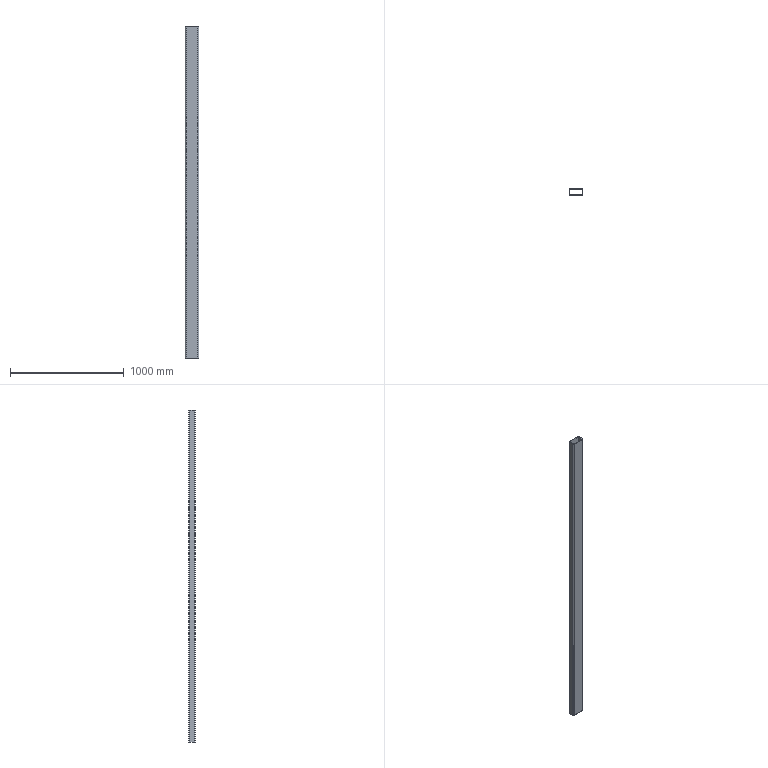Part | SolidWorks | features Extrusion 1 | 1 solid | 18 faces | box 120 x 60 x 2920 mm | volume 4776009 mm3 | plane 10 | cylinder 8 | commonest cylinder face diameters 10 x4 20 x4
STEP:
#1=CARTESIAN_POINT('',(110.,0.,2920.));
#2=VERTEX_POINT('',#1);
#3=CARTESIAN_POINT('',(120.,10.,2920.));
#4=VERTEX_POINT('',#3);
#5=CARTESIAN_POINT('',(110.,10.,2920.));
#6=DIRECTION('',(0.,0.,1.));
#7=DIRECTION('',(-1.,0.,0.));
#8=AXIS2_PLACEMENT_3D('',#5,#6,#7);
#9=CIRCLE('',#8,10.);
#10=EDGE_CURVE('',#2,#4,#9,.T.);
#11=ORIENTED_EDGE('',*,*,#10,.T.);
#12=CARTESIAN_POINT('',(120.,50.,2920.));
#13=VERTEX_POINT('',#12);
#14=CARTESIAN_POINT('',(120.,10.,2920.));
#15=DIRECTION('',(0.,1.,0.));
#16=VECTOR('',#15,1000.);
#17=LINE('',#14,#16);
#18=EDGE_CURVE('',#4,#13,#17,.T.);
#19=ORIENTED_EDGE('',*,*,#18,.T.);
#20=CARTESIAN_POINT('',(110.,60.,2920.));
#21=VERTEX_POINT('',#20);
#22=CARTESIAN_POINT('',(110.,50.,2920.));
#23=DIRECTION('',(0.,0.,1.));
#24=DIRECTION('',(1.,0.,0.));
#25=AXIS2_PLACEMENT_3D('',#22,#23,#24);
#26=CIRCLE('',#25,10.);
#27=EDGE_CURVE('',#13,#21,#26,.T.);
#28=ORIENTED_EDGE('',*,*,#27,.T.);
#29=CARTESIAN_POINT('',(10.,60.,2920.));
#30=VERTEX_POINT('',#29);
#31=CARTESIAN_POINT('',(10.,60.,2920.));
#32=DIRECTION('',(-1.,0.,0.));
#33=VECTOR('',#32,1000.);
#34=LINE('',#31,#33);
#35=EDGE_CURVE('',#21,#30,#34,.T.);
#36=ORIENTED_EDGE('',*,*,#35,.T.);
#37=CARTESIAN_POINT('',(0.,50.,2920.));
#38=VERTEX_POINT('',#37);
#39=CARTESIAN_POINT('',(10.,50.,2920.));
#40=DIRECTION('',(0.,0.,1.));
#41=DIRECTION('',(-1.,0.,0.));
#42=AXIS2_PLACEMENT_3D('',#39,#40,#41);
#43=CIRCLE('',#42,10.);
#44=EDGE_CURVE('',#30,#38,#43,.T.);
#45=ORIENTED_EDGE('',*,*,#44,.T.);
#46=CARTESIAN_POINT('',(0.,10.,2920.));
#47=VERTEX_POINT('',#46);
#48=CARTESIAN_POINT('',(0.,10.,2920.));
#49=DIRECTION('',(0.,-1.,0.));
#50=VECTOR('',#49,1000.);
#51=LINE('',#48,#50);
#52=EDGE_CURVE('',#38,#47,#51,.T.);
#53=ORIENTED_EDGE('',*,*,#52,.T.);
#54=CARTESIAN_POINT('',(10.,0.,2920.));
#55=VERTEX_POINT('',#54);
#56=CARTESIAN_POINT('',(10.,10.,2920.));
#57=DIRECTION('',(0.,0.,1.));
#58=DIRECTION('',(-1.,0.,0.));
#59=AXIS2_PLACEMENT_3D('',#56,#57,#58);
#60=CIRCLE('',#59,10.);
#61=EDGE_CURVE('',#47,#55,#60,.T.);
#62=ORIENTED_EDGE('',*,*,#61,.T.);
#63=CARTESIAN_POINT('',(10.,0.,2920.));
#64=DIRECTION('',(1.,0.,0.));
#65=VECTOR('',#64,1000.);
#66=LINE('',#63,#65);
#67=EDGE_CURVE('',#55,#2,#66,.T.);
#68=ORIENTED_EDGE('',*,*,#67,.T.);
#69=EDGE_LOOP('',(#11,#19,#28,#36,#45,#53,#62,#68));
#70=FACE_OUTER_BOUND('',#69,.T.);
#71=CARTESIAN_POINT('',(10.,55.,2920.));
#72=VERTEX_POINT('',#71);
#73=CARTESIAN_POINT('',(5.,50.,2920.));
#74=VERTEX_POINT('',#73);
#75=CARTESIAN_POINT('',(10.,50.,2920.));
#76=DIRECTION('',(0.,0.,1.));
#77=DIRECTION('',(-1.,0.,0.));
#78=AXIS2_PLACEMENT_3D('',#75,#76,#77);
#79=CIRCLE('',#78,5.);
#80=EDGE_CURVE('',#72,#74,#79,.T.);
#81=ORIENTED_EDGE('',*,*,#80,.F.);
#82=CARTESIAN_POINT('',(110.,55.,2920.));
#83=VERTEX_POINT('',#82);
#84=CARTESIAN_POINT('',(10.,55.,2920.));
#85=DIRECTION('',(-1.,0.,0.));
#86=VECTOR('',#85,1000.);
#87=LINE('',#84,#86);
#88=EDGE_CURVE('',#83,#72,#87,.T.);
#89=ORIENTED_EDGE('',*,*,#88,.F.);
#90=CARTESIAN_POINT('',(115.,50.,2920.));
#91=VERTEX_POINT('',#90);
#92=CARTESIAN_POINT('',(110.,50.,2920.));
#93=DIRECTION('',(0.,0.,1.));
#94=DIRECTION('',(1.,0.,0.));
#95=AXIS2_PLACEMENT_3D('',#92,#93,#94);
#96=CIRCLE('',#95,5.);
#97=EDGE_CURVE('',#91,#83,#96,.T.);
#98=ORIENTED_EDGE('',*,*,#97,.F.);
#99=CARTESIAN_POINT('',(115.,10.,2920.));
#100=VERTEX_POINT('',#99);
#101=CARTESIAN_POINT('',(115.,10.,2920.));
#102=DIRECTION('',(0.,1.,0.));
#103=VECTOR('',#102,1000.);
#104=LINE('',#101,#103);
#105=EDGE_CURVE('',#100,#91,#104,.T.);
#106=ORIENTED_EDGE('',*,*,#105,.F.);
#107=CARTESIAN_POINT('',(110.,5.,2920.));
#108=VERTEX_POINT('',#107);
#109=CARTESIAN_POINT('',(110.,10.,2920.));
#110=DIRECTION('',(0.,0.,1.));
#111=DIRECTION('',(-1.,0.,0.));
#112=AXIS2_PLACEMENT_3D('',#109,#110,#111);
#113=CIRCLE('',#112,5.);
#114=EDGE_CURVE('',#108,#100,#113,.T.);
#115=ORIENTED_EDGE('',*,*,#114,.F.);
#116=CARTESIAN_POINT('',(10.,5.,2920.));
#117=VERTEX_POINT('',#116);
#118=CARTESIAN_POINT('',(10.,5.,2920.));
#119=DIRECTION('',(1.,0.,0.));
#120=VECTOR('',#119,1000.);
#121=LINE('',#118,#120);
#122=EDGE_CURVE('',#117,#108,#121,.T.);
#123=ORIENTED_EDGE('',*,*,#122,.F.);
#124=CARTESIAN_POINT('',(5.,10.,2920.));
#125=VERTEX_POINT('',#124);
#126=CARTESIAN_POINT('',(10.,10.,2920.));
#127=DIRECTION('',(0.,0.,1.));
#128=DIRECTION('',(-1.,0.,0.));
#129=AXIS2_PLACEMENT_3D('',#126,#127,#128);
#130=CIRCLE('',#129,5.);
#131=EDGE_CURVE('',#125,#117,#130,.T.);
#132=ORIENTED_EDGE('',*,*,#131,.F.);
#133=CARTESIAN_POINT('',(5.,10.,2920.));
#134=DIRECTION('',(0.,-1.,0.));
#135=VECTOR('',#134,1000.);
#136=LINE('',#133,#135);
#137=EDGE_CURVE('',#74,#125,#136,.T.);
#138=ORIENTED_EDGE('',*,*,#137,.F.);
#139=EDGE_LOOP('',(#81,#89,#98,#106,#115,#123,#132,#138));
#140=FACE_BOUND('',#139,.T.);
#141=CARTESIAN_POINT('',(110.,10.,2920.));
#142=DIRECTION('',(0.,0.,-1.));
#143=DIRECTION('',(-1.,0.,0.));
#144=AXIS2_PLACEMENT_3D('',#141,#142,#143);
#145=PLANE('',#144);
#146=ADVANCED_FACE('',(#70,#140),#145,.F.);
#147=CARTESIAN_POINT('',(110.,0.,0.));
#148=VERTEX_POINT('',#147);
#149=CARTESIAN_POINT('',(120.,10.,0.));
#150=VERTEX_POINT('',#149);
#151=CARTESIAN_POINT('',(110.,10.,0.));
#152=DIRECTION('',(0.,0.,1.));
#153=DIRECTION('',(-1.,0.,0.));
#154=AXIS2_PLACEMENT_3D('',#151,#152,#153);
#155=CIRCLE('',#154,10.);
#156=EDGE_CURVE('',#148,#150,#155,.T.);
#157=ORIENTED_EDGE('',*,*,#156,.F.);
#158=CARTESIAN_POINT('',(10.,0.,0.));
#159=VERTEX_POINT('',#158);
#160=CARTESIAN_POINT('',(10.,0.,0.));
#161=DIRECTION('',(1.,0.,0.));
#162=VECTOR('',#161,1000.);
#163=LINE('',#160,#162);
#164=EDGE_CURVE('',#159,#148,#163,.T.);
#165=ORIENTED_EDGE('',*,*,#164,.F.);
#166=CARTESIAN_POINT('',(0.,10.,0.));
#167=VERTEX_POINT('',#166);
#168=CARTESIAN_POINT('',(10.,10.,0.));
#169=DIRECTION('',(0.,0.,1.));
#170=DIRECTION('',(-1.,0.,0.));
#171=AXIS2_PLACEMENT_3D('',#168,#169,#170);
#172=CIRCLE('',#171,10.);
#173=EDGE_CURVE('',#167,#159,#172,.T.);
#174=ORIENTED_EDGE('',*,*,#173,.F.);
#175=CARTESIAN_POINT('',(0.,50.,0.));
#176=VERTEX_POINT('',#175);
#177=CARTESIAN_POINT('',(0.,10.,0.));
#178=DIRECTION('',(0.,-1.,0.));
#179=VECTOR('',#178,1000.);
#180=LINE('',#177,#179);
#181=EDGE_CURVE('',#176,#167,#180,.T.);
#182=ORIENTED_EDGE('',*,*,#181,.F.);
#183=CARTESIAN_POINT('',(10.,60.,0.));
#184=VERTEX_POINT('',#183);
#185=CARTESIAN_POINT('',(10.,50.,0.));
#186=DIRECTION('',(0.,0.,1.));
#187=DIRECTION('',(-1.,0.,0.));
#188=AXIS2_PLACEMENT_3D('',#185,#186,#187);
#189=CIRCLE('',#188,10.);
#190=EDGE_CURVE('',#184,#176,#189,.T.);
#191=ORIENTED_EDGE('',*,*,#190,.F.);
#192=CARTESIAN_POINT('',(110.,60.,0.));
#193=VERTEX_POINT('',#192);
#194=CARTESIAN_POINT('',(10.,60.,0.));
#195=DIRECTION('',(-1.,0.,0.));
#196=VECTOR('',#195,1000.);
#197=LINE('',#194,#196);
#198=EDGE_CURVE('',#193,#184,#197,.T.);
#199=ORIENTED_EDGE('',*,*,#198,.F.);
#200=CARTESIAN_POINT('',(120.,50.,0.));
#201=VERTEX_POINT('',#200);
#202=CARTESIAN_POINT('',(110.,50.,0.));
#203=DIRECTION('',(0.,0.,1.));
#204=DIRECTION('',(1.,0.,0.));
#205=AXIS2_PLACEMENT_3D('',#202,#203,#204);
#206=CIRCLE('',#205,10.);
#207=EDGE_CURVE('',#201,#193,#206,.T.);
#208=ORIENTED_EDGE('',*,*,#207,.F.);
#209=CARTESIAN_POINT('',(120.,10.,0.));
#210=DIRECTION('',(0.,1.,0.));
#211=VECTOR('',#210,1000.);
#212=LINE('',#209,#211);
#213=EDGE_CURVE('',#150,#201,#212,.T.);
#214=ORIENTED_EDGE('',*,*,#213,.F.);
#215=EDGE_LOOP('',(#157,#165,#174,#182,#191,#199,#208,#214));
#216=FACE_OUTER_BOUND('',#215,.T.);
#217=CARTESIAN_POINT('',(110.,55.,0.));
#218=VERTEX_POINT('',#217);
#219=CARTESIAN_POINT('',(10.,55.,0.));
#220=VERTEX_POINT('',#219);
#221=CARTESIAN_POINT('',(10.,55.,0.));
#222=DIRECTION('',(-1.,0.,0.));
#223=VECTOR('',#222,1000.);
#224=LINE('',#221,#223);
#225=EDGE_CURVE('',#218,#220,#224,.T.);
#226=ORIENTED_EDGE('',*,*,#225,.T.);
#227=CARTESIAN_POINT('',(5.,50.,0.));
#228=VERTEX_POINT('',#227);
#229=CARTESIAN_POINT('',(10.,50.,0.));
#230=DIRECTION('',(0.,0.,1.));
#231=DIRECTION('',(-1.,0.,0.));
#232=AXIS2_PLACEMENT_3D('',#229,#230,#231);
#233=CIRCLE('',#232,5.);
#234=EDGE_CURVE('',#220,#228,#233,.T.);
#235=ORIENTED_EDGE('',*,*,#234,.T.);
#236=CARTESIAN_POINT('',(5.,10.,0.));
#237=VERTEX_POINT('',#236);
#238=CARTESIAN_POINT('',(5.,10.,0.));
#239=DIRECTION('',(0.,-1.,0.));
#240=VECTOR('',#239,1000.);
#241=LINE('',#238,#240);
#242=EDGE_CURVE('',#228,#237,#241,.T.);
#243=ORIENTED_EDGE('',*,*,#242,.T.);
#244=CARTESIAN_POINT('',(10.,5.,0.));
#245=VERTEX_POINT('',#244);
#246=CARTESIAN_POINT('',(10.,10.,0.));
#247=DIRECTION('',(0.,0.,1.));
#248=DIRECTION('',(-1.,0.,0.));
#249=AXIS2_PLACEMENT_3D('',#246,#247,#248);
#250=CIRCLE('',#249,5.);
#251=EDGE_CURVE('',#237,#245,#250,.T.);
#252=ORIENTED_EDGE('',*,*,#251,.T.);
#253=CARTESIAN_POINT('',(110.,5.,0.));
#254=VERTEX_POINT('',#253);
#255=CARTESIAN_POINT('',(10.,5.,0.));
#256=DIRECTION('',(1.,0.,0.));
#257=VECTOR('',#256,1000.);
#258=LINE('',#255,#257);
#259=EDGE_CURVE('',#245,#254,#258,.T.);
#260=ORIENTED_EDGE('',*,*,#259,.T.);
#261=CARTESIAN_POINT('',(115.,10.,0.));
#262=VERTEX_POINT('',#261);
#263=CARTESIAN_POINT('',(110.,10.,0.));
#264=DIRECTION('',(0.,0.,1.));
#265=DIRECTION('',(-1.,0.,0.));
#266=AXIS2_PLACEMENT_3D('',#263,#264,#265);
#267=CIRCLE('',#266,5.);
#268=EDGE_CURVE('',#254,#262,#267,.T.);
#269=ORIENTED_EDGE('',*,*,#268,.T.);
#270=CARTESIAN_POINT('',(115.,50.,0.));
#271=VERTEX_POINT('',#270);
#272=CARTESIAN_POINT('',(115.,10.,0.));
#273=DIRECTION('',(0.,1.,0.));
#274=VECTOR('',#273,1000.);
#275=LINE('',#272,#274);
#276=EDGE_CURVE('',#262,#271,#275,.T.);
#277=ORIENTED_EDGE('',*,*,#276,.T.);
#278=CARTESIAN_POINT('',(110.,50.,0.));
#279=DIRECTION('',(0.,0.,1.));
#280=DIRECTION('',(1.,0.,0.));
#281=AXIS2_PLACEMENT_3D('',#278,#279,#280);
#282=CIRCLE('',#281,5.);
#283=EDGE_CURVE('',#271,#218,#282,.T.);
#284=ORIENTED_EDGE('',*,*,#283,.T.);
#285=EDGE_LOOP('',(#226,#235,#243,#252,#260,#269,#277,#284));
#286=FACE_BOUND('',#285,.T.);
#287=CARTESIAN_POINT('',(110.,10.,0.));
#288=DIRECTION('',(0.,0.,-1.));
#289=DIRECTION('',(-1.,0.,0.));
#290=AXIS2_PLACEMENT_3D('',#287,#288,#289);
#291=PLANE('',#290);
#292=ADVANCED_FACE('',(#216,#286),#291,.T.);
#293=ORIENTED_EDGE('',*,*,#156,.T.);
#294=CARTESIAN_POINT('',(120.,10.,2920.));
#295=DIRECTION('',(0.,0.,-1.));
#296=VECTOR('',#295,1000.);
#297=LINE('',#294,#296);
#298=EDGE_CURVE('',#4,#150,#297,.T.);
#299=ORIENTED_EDGE('',*,*,#298,.F.);
#300=ORIENTED_EDGE('',*,*,#10,.F.);
#301=CARTESIAN_POINT('',(110.,0.,2920.));
#302=DIRECTION('',(0.,0.,-1.));
#303=VECTOR('',#302,1000.);
#304=LINE('',#301,#303);
#305=EDGE_CURVE('',#2,#148,#304,.T.);
#306=ORIENTED_EDGE('',*,*,#305,.T.);
#307=EDGE_LOOP('',(#293,#299,#300,#306));
#308=FACE_OUTER_BOUND('',#307,.T.);
#309=CARTESIAN_POINT('',(110.,10.,2920.));
#310=DIRECTION('',(0.,0.,-1.));
#311=DIRECTION('',(-1.,0.,0.));
#312=AXIS2_PLACEMENT_3D('',#309,#310,#311);
#313=CYLINDRICAL_SURFACE('',#312,10.);
#314=ADVANCED_FACE('',(#308),#313,.T.);
#315=ORIENTED_EDGE('',*,*,#213,.T.);
#316=CARTESIAN_POINT('',(120.,50.,2920.));
#317=DIRECTION('',(0.,0.,-1.));
#318=VECTOR('',#317,1000.);
#319=LINE('',#316,#318);
#320=EDGE_CURVE('',#13,#201,#319,.T.);
#321=ORIENTED_EDGE('',*,*,#320,.F.);
#322=ORIENTED_EDGE('',*,*,#18,.F.);
#323=ORIENTED_EDGE('',*,*,#298,.T.);
#324=EDGE_LOOP('',(#315,#321,#322,#323));
#325=FACE_OUTER_BOUND('',#324,.T.);
#326=CARTESIAN_POINT('',(120.,10.,2920.));
#327=DIRECTION('',(-1.,0.,0.));
#328=DIRECTION('',(0.,-1.,0.));
#329=AXIS2_PLACEMENT_3D('',#326,#327,#328);
#330=PLANE('',#329);
#331=ADVANCED_FACE('',(#325),#330,.F.);
#332=ORIENTED_EDGE('',*,*,#207,.T.);
#333=CARTESIAN_POINT('',(110.,60.,2920.));
#334=DIRECTION('',(0.,0.,-1.));
#335=VECTOR('',#334,1000.);
#336=LINE('',#333,#335);
#337=EDGE_CURVE('',#21,#193,#336,.T.);
#338=ORIENTED_EDGE('',*,*,#337,.F.);
#339=ORIENTED_EDGE('',*,*,#27,.F.);
#340=ORIENTED_EDGE('',*,*,#320,.T.);
#341=EDGE_LOOP('',(#332,#338,#339,#340));
#342=FACE_OUTER_BOUND('',#341,.T.);
#343=CARTESIAN_POINT('',(110.,50.,2920.));
#344=DIRECTION('',(0.,0.,-1.));
#345=DIRECTION('',(-1.,0.,0.));
#346=AXIS2_PLACEMENT_3D('',#343,#344,#345);
#347=CYLINDRICAL_SURFACE('',#346,10.);
#348=ADVANCED_FACE('',(#342),#347,.T.);
#349=ORIENTED_EDGE('',*,*,#198,.T.);
#350=CARTESIAN_POINT('',(10.,60.,2920.));
#351=DIRECTION('',(0.,0.,-1.));
#352=VECTOR('',#351,1000.);
#353=LINE('',#350,#352);
#354=EDGE_CURVE('',#30,#184,#353,.T.);
#355=ORIENTED_EDGE('',*,*,#354,.F.);
#356=ORIENTED_EDGE('',*,*,#35,.F.);
#357=ORIENTED_EDGE('',*,*,#337,.T.);
#358=EDGE_LOOP('',(#349,#355,#356,#357));
#359=FACE_OUTER_BOUND('',#358,.T.);
#360=CARTESIAN_POINT('',(10.,60.,2920.));
#361=DIRECTION('',(0.,-1.,0.));
#362=DIRECTION('',(0.,0.,-1.));
#363=AXIS2_PLACEMENT_3D('',#360,#361,#362);
#364=PLANE('',#363);
#365=ADVANCED_FACE('',(#359),#364,.F.);
#366=ORIENTED_EDGE('',*,*,#190,.T.);
#367=CARTESIAN_POINT('',(0.,50.,2920.));
#368=DIRECTION('',(0.,0.,-1.));
#369=VECTOR('',#368,1000.);
#370=LINE('',#367,#369);
#371=EDGE_CURVE('',#38,#176,#370,.T.);
#372=ORIENTED_EDGE('',*,*,#371,.F.);
#373=ORIENTED_EDGE('',*,*,#44,.F.);
#374=ORIENTED_EDGE('',*,*,#354,.T.);
#375=EDGE_LOOP('',(#366,#372,#373,#374));
#376=FACE_OUTER_BOUND('',#375,.T.);
#377=CARTESIAN_POINT('',(10.,50.,2920.));
#378=DIRECTION('',(0.,0.,-1.));
#379=DIRECTION('',(-1.,0.,0.));
#380=AXIS2_PLACEMENT_3D('',#377,#378,#379);
#381=CYLINDRICAL_SURFACE('',#380,10.);
#382=ADVANCED_FACE('',(#376),#381,.T.);
#383=ORIENTED_EDGE('',*,*,#181,.T.);
#384=CARTESIAN_POINT('',(0.,10.,2920.));
#385=DIRECTION('',(0.,0.,-1.));
#386=VECTOR('',#385,1000.);
#387=LINE('',#384,#386);
#388=EDGE_CURVE('',#47,#167,#387,.T.);
#389=ORIENTED_EDGE('',*,*,#388,.F.);
#390=ORIENTED_EDGE('',*,*,#52,.F.);
#391=ORIENTED_EDGE('',*,*,#371,.T.);
#392=EDGE_LOOP('',(#383,#389,#390,#391));
#393=FACE_OUTER_BOUND('',#392,.T.);
#394=CARTESIAN_POINT('',(0.,10.,2920.));
#395=DIRECTION('',(1.,0.,0.));
#396=DIRECTION('',(0.,1.,0.));
#397=AXIS2_PLACEMENT_3D('',#394,#395,#396);
#398=PLANE('',#397);
#399=ADVANCED_FACE('',(#393),#398,.F.);
#400=ORIENTED_EDGE('',*,*,#173,.T.);
#401=CARTESIAN_POINT('',(10.,0.,2920.));
#402=DIRECTION('',(0.,0.,-1.));
#403=VECTOR('',#402,1000.);
#404=LINE('',#401,#403);
#405=EDGE_CURVE('',#55,#159,#404,.T.);
#406=ORIENTED_EDGE('',*,*,#405,.F.);
#407=ORIENTED_EDGE('',*,*,#61,.F.);
#408=ORIENTED_EDGE('',*,*,#388,.T.);
#409=EDGE_LOOP('',(#400,#406,#407,#408));
#410=FACE_OUTER_BOUND('',#409,.T.);
#411=CARTESIAN_POINT('',(10.,10.,2920.));
#412=DIRECTION('',(0.,0.,-1.));
#413=DIRECTION('',(-1.,0.,0.));
#414=AXIS2_PLACEMENT_3D('',#411,#412,#413);
#415=CYLINDRICAL_SURFACE('',#414,10.);
#416=ADVANCED_FACE('',(#410),#415,.T.);
#417=ORIENTED_EDGE('',*,*,#164,.T.);
#418=ORIENTED_EDGE('',*,*,#305,.F.);
#419=ORIENTED_EDGE('',*,*,#67,.F.);
#420=ORIENTED_EDGE('',*,*,#405,.T.);
#421=EDGE_LOOP('',(#417,#418,#419,#420));
#422=FACE_OUTER_BOUND('',#421,.T.);
#423=CARTESIAN_POINT('',(10.,0.,2920.));
#424=DIRECTION('',(0.,1.,0.));
#425=DIRECTION('',(0.,0.,1.));
#426=AXIS2_PLACEMENT_3D('',#423,#424,#425);
#427=PLANE('',#426);
#428=ADVANCED_FACE('',(#422),#427,.F.);
#429=ORIENTED_EDGE('',*,*,#234,.F.);
#430=CARTESIAN_POINT('',(10.,55.,2920.));
#431=DIRECTION('',(0.,0.,-1.));
#432=VECTOR('',#431,1000.);
#433=LINE('',#430,#432);
#434=EDGE_CURVE('',#72,#220,#433,.T.);
#435=ORIENTED_EDGE('',*,*,#434,.F.);
#436=ORIENTED_EDGE('',*,*,#80,.T.);
#437=CARTESIAN_POINT('',(5.,50.,2920.));
#438=DIRECTION('',(0.,0.,-1.));
#439=VECTOR('',#438,1000.);
#440=LINE('',#437,#439);
#441=EDGE_CURVE('',#74,#228,#440,.T.);
#442=ORIENTED_EDGE('',*,*,#441,.T.);
#443=EDGE_LOOP('',(#429,#435,#436,#442));
#444=FACE_OUTER_BOUND('',#443,.T.);
#445=CARTESIAN_POINT('',(10.,50.,2920.));
#446=DIRECTION('',(0.,0.,-1.));
#447=DIRECTION('',(-1.,0.,0.));
#448=AXIS2_PLACEMENT_3D('',#445,#446,#447);
#449=CYLINDRICAL_SURFACE('',#448,5.);
#450=ADVANCED_FACE('',(#444),#449,.F.);
#451=ORIENTED_EDGE('',*,*,#242,.F.);
#452=ORIENTED_EDGE('',*,*,#441,.F.);
#453=ORIENTED_EDGE('',*,*,#137,.T.);
#454=CARTESIAN_POINT('',(5.,10.,2920.));
#455=DIRECTION('',(0.,0.,-1.));
#456=VECTOR('',#455,1000.);
#457=LINE('',#454,#456);
#458=EDGE_CURVE('',#125,#237,#457,.T.);
#459=ORIENTED_EDGE('',*,*,#458,.T.);
#460=EDGE_LOOP('',(#451,#452,#453,#459));
#461=FACE_OUTER_BOUND('',#460,.T.);
#462=CARTESIAN_POINT('',(5.,10.,2920.));
#463=DIRECTION('',(1.,0.,0.));
#464=DIRECTION('',(0.,1.,0.));
#465=AXIS2_PLACEMENT_3D('',#462,#463,#464);
#466=PLANE('',#465);
#467=ADVANCED_FACE('',(#461),#466,.T.);
#468=ORIENTED_EDGE('',*,*,#251,.F.);
#469=ORIENTED_EDGE('',*,*,#458,.F.);
#470=ORIENTED_EDGE('',*,*,#131,.T.);
#471=CARTESIAN_POINT('',(10.,5.,2920.));
#472=DIRECTION('',(0.,0.,-1.));
#473=VECTOR('',#472,1000.);
#474=LINE('',#471,#473);
#475=EDGE_CURVE('',#117,#245,#474,.T.);
#476=ORIENTED_EDGE('',*,*,#475,.T.);
#477=EDGE_LOOP('',(#468,#469,#470,#476));
#478=FACE_OUTER_BOUND('',#477,.T.);
#479=CARTESIAN_POINT('',(10.,10.,2920.));
#480=DIRECTION('',(0.,0.,-1.));
#481=DIRECTION('',(-1.,0.,0.));
#482=AXIS2_PLACEMENT_3D('',#479,#480,#481);
#483=CYLINDRICAL_SURFACE('',#482,5.);
#484=ADVANCED_FACE('',(#478),#483,.F.);
#485=ORIENTED_EDGE('',*,*,#259,.F.);
#486=ORIENTED_EDGE('',*,*,#475,.F.);
#487=ORIENTED_EDGE('',*,*,#122,.T.);
#488=CARTESIAN_POINT('',(110.,5.,2920.));
#489=DIRECTION('',(0.,0.,-1.));
#490=VECTOR('',#489,1000.);
#491=LINE('',#488,#490);
#492=EDGE_CURVE('',#108,#254,#491,.T.);
#493=ORIENTED_EDGE('',*,*,#492,.T.);
#494=EDGE_LOOP('',(#485,#486,#487,#493));
#495=FACE_OUTER_BOUND('',#494,.T.);
#496=CARTESIAN_POINT('',(10.,5.,2920.));
#497=DIRECTION('',(0.,1.,0.));
#498=DIRECTION('',(0.,0.,1.));
#499=AXIS2_PLACEMENT_3D('',#496,#497,#498);
#500=PLANE('',#499);
#501=ADVANCED_FACE('',(#495),#500,.T.);
#502=ORIENTED_EDGE('',*,*,#268,.F.);
#503=ORIENTED_EDGE('',*,*,#492,.F.);
#504=ORIENTED_EDGE('',*,*,#114,.T.);
#505=CARTESIAN_POINT('',(115.,10.,2920.));
#506=DIRECTION('',(0.,0.,-1.));
#507=VECTOR('',#506,1000.);
#508=LINE('',#505,#507);
#509=EDGE_CURVE('',#100,#262,#508,.T.);
#510=ORIENTED_EDGE('',*,*,#509,.T.);
#511=EDGE_LOOP('',(#502,#503,#504,#510));
#512=FACE_OUTER_BOUND('',#511,.T.);
#513=CARTESIAN_POINT('',(110.,10.,2920.));
#514=DIRECTION('',(0.,0.,-1.));
#515=DIRECTION('',(-1.,0.,0.));
#516=AXIS2_PLACEMENT_3D('',#513,#514,#515);
#517=CYLINDRICAL_SURFACE('',#516,5.);
#518=ADVANCED_FACE('',(#512),#517,.F.);
#519=ORIENTED_EDGE('',*,*,#276,.F.);
#520=ORIENTED_EDGE('',*,*,#509,.F.);
#521=ORIENTED_EDGE('',*,*,#105,.T.);
#522=CARTESIAN_POINT('',(115.,50.,2920.));
#523=DIRECTION('',(0.,0.,-1.));
#524=VECTOR('',#523,1000.);
#525=LINE('',#522,#524);
#526=EDGE_CURVE('',#91,#271,#525,.T.);
#527=ORIENTED_EDGE('',*,*,#526,.T.);
#528=EDGE_LOOP('',(#519,#520,#521,#527));
#529=FACE_OUTER_BOUND('',#528,.T.);
#530=CARTESIAN_POINT('',(115.,10.,2920.));
#531=DIRECTION('',(-1.,0.,0.));
#532=DIRECTION('',(0.,0.,1.));
#533=AXIS2_PLACEMENT_3D('',#530,#531,#532);
#534=PLANE('',#533);
#535=ADVANCED_FACE('',(#529),#534,.T.);
#536=ORIENTED_EDGE('',*,*,#283,.F.);
#537=ORIENTED_EDGE('',*,*,#526,.F.);
#538=ORIENTED_EDGE('',*,*,#97,.T.);
#539=CARTESIAN_POINT('',(110.,55.,2920.));
#540=DIRECTION('',(0.,0.,-1.));
#541=VECTOR('',#540,1000.);
#542=LINE('',#539,#541);
#543=EDGE_CURVE('',#83,#218,#542,.T.);
#544=ORIENTED_EDGE('',*,*,#543,.T.);
#545=EDGE_LOOP('',(#536,#537,#538,#544));
#546=FACE_OUTER_BOUND('',#545,.T.);
#547=CARTESIAN_POINT('',(110.,50.,2920.));
#548=DIRECTION('',(0.,0.,-1.));
#549=DIRECTION('',(-1.,0.,0.));
#550=AXIS2_PLACEMENT_3D('',#547,#548,#549);
#551=CYLINDRICAL_SURFACE('',#550,5.);
#552=ADVANCED_FACE('',(#546),#551,.F.);
#553=ORIENTED_EDGE('',*,*,#225,.F.);
#554=ORIENTED_EDGE('',*,*,#543,.F.);
#555=ORIENTED_EDGE('',*,*,#88,.T.);
#556=ORIENTED_EDGE('',*,*,#434,.T.);
#557=EDGE_LOOP('',(#553,#554,#555,#556));
#558=FACE_OUTER_BOUND('',#557,.T.);
#559=CARTESIAN_POINT('',(10.,55.,2920.));
#560=DIRECTION('',(0.,-1.,0.));
#561=DIRECTION('',(0.,0.,-1.));
#562=AXIS2_PLACEMENT_3D('',#559,#560,#561);
#563=PLANE('',#562);
#564=ADVANCED_FACE('',(#558),#563,.T.);
#565=CLOSED_SHELL('',(#146,#292,#314,#331,#348,#365,#382,#399,#416,#428,#450,#467,#484,#501,#518,#535,#552,#564));
#566=MANIFOLD_SOLID_BREP('',#565);
#567=CARTESIAN_POINT('',(0.,0.,0.));
#568=DIRECTION('',(0.,0.,1.));
#569=DIRECTION('',(1.,0.,0.));
#570=AXIS2_PLACEMENT_3D('',#567,#568,#569);
#571=(LENGTH_UNIT()NAMED_UNIT(*)SI_UNIT(.MILLI.,.METRE.));
#572=UNCERTAINTY_MEASURE_WITH_UNIT(LENGTH_MEASURE(0.00001),#571,'','');
#573=(NAMED_UNIT(*)PLANE_ANGLE_UNIT()SI_UNIT($,.RADIAN.));
#574=(NAMED_UNIT(*)SI_UNIT($,.STERADIAN.)SOLID_ANGLE_UNIT());
#575=(GEOMETRIC_REPRESENTATION_CONTEXT(3)GLOBAL_UNCERTAINTY_ASSIGNED_CONTEXT((#572))GLOBAL_UNIT_ASSIGNED_CONTEXT((#571,#573,#574))REPRESENTATION_CONTEXT('',''));
#576=ADVANCED_BREP_SHAPE_REPRESENTATION('',(#566,#570),#575);